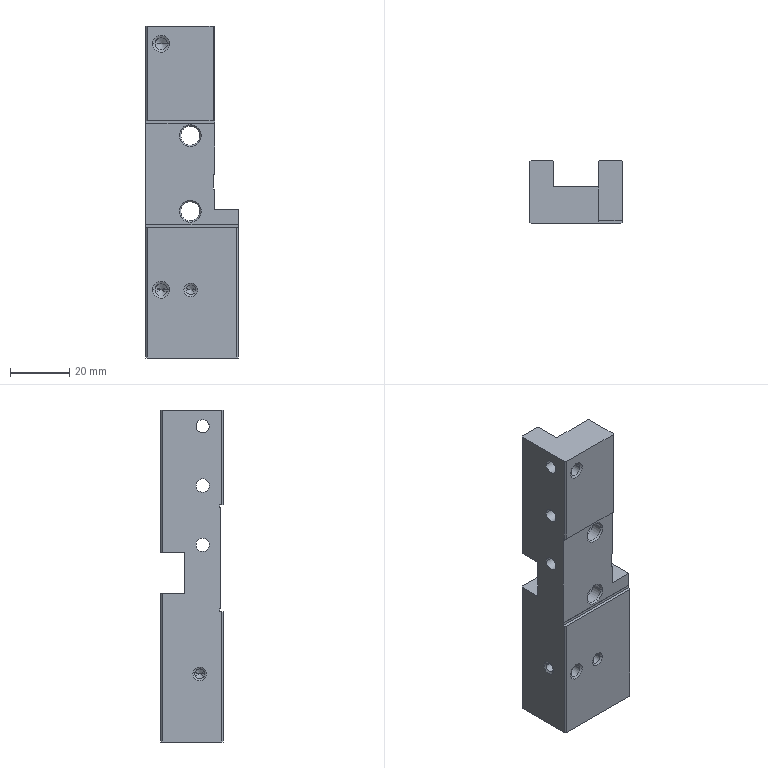Part | NX | 1 solid | 132 faces | box 31.2 x 21.2 x 112 mm | volume 42736 mm3 | cone 52 | plane 40 | cylinder 40 | commonest cylinder face diameters 3.3 x12 2.5 x8 4.5 x7 4.2 x5 6.4 x4 11 x4